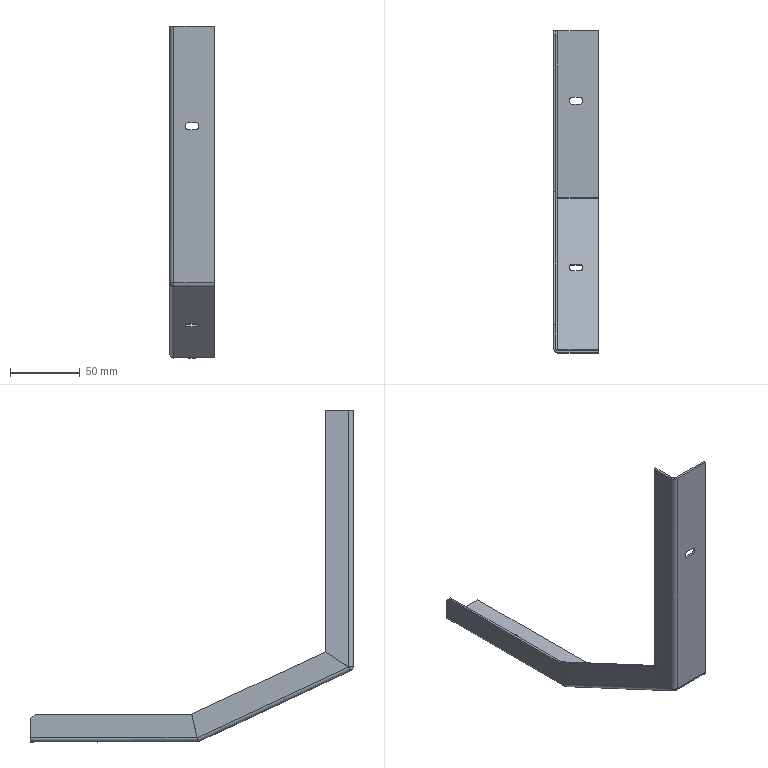Part | NX | features solid 2 | 1 solid | 51 faces | box 32 x 231 x 238 mm | volume 31049 mm3 | plane 31 | cylinder 16 | spline 4 | commonest cylinder face diameters 5 x6 3 x5 6 x5